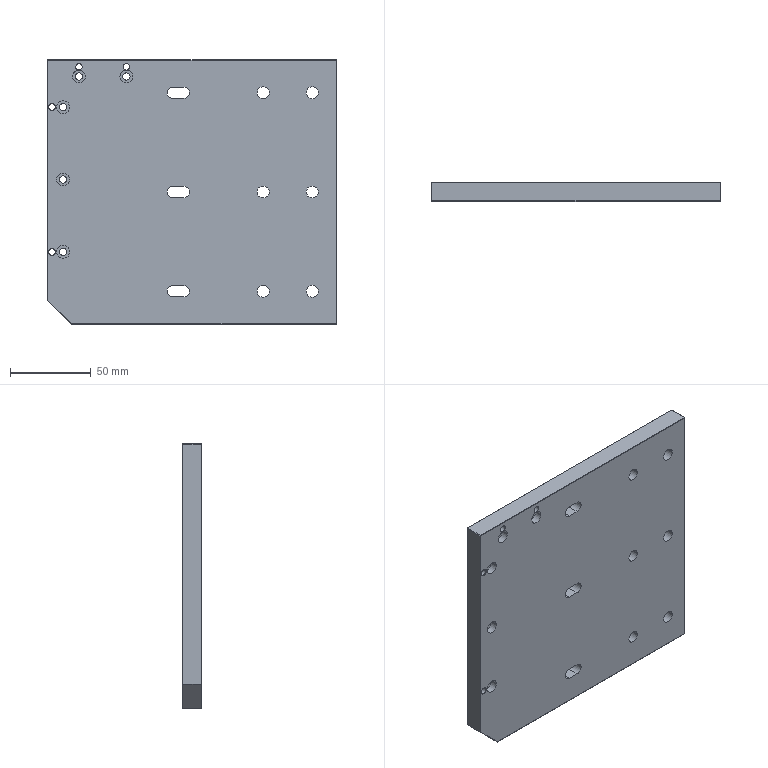Part | NX | 1 solid | 96 faces | box 180 x 12 x 164.5 mm | volume 345268 mm3 | cylinder 49 | plane 31 | cone 16 | commonest cylinder face diameters 7.5 x12 4.5 x10 8 x10 7 x9 4 x8